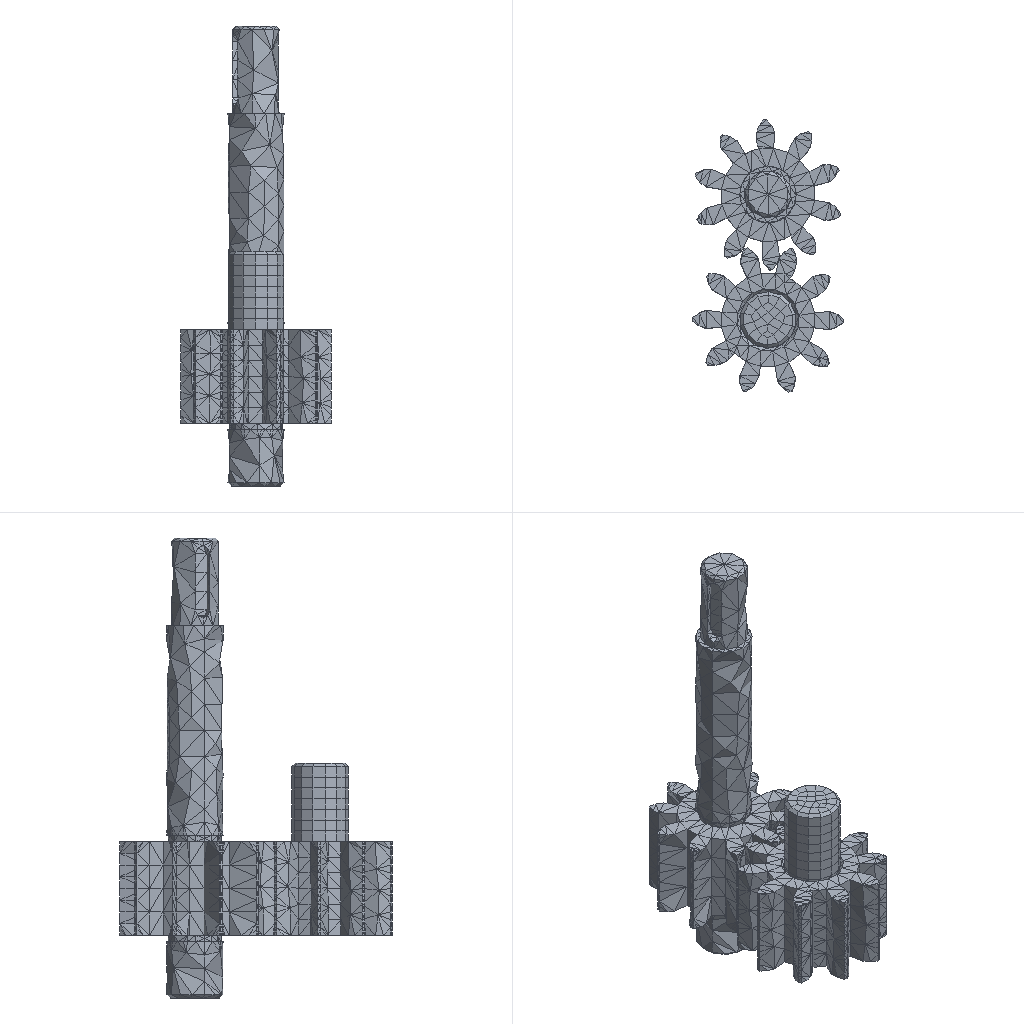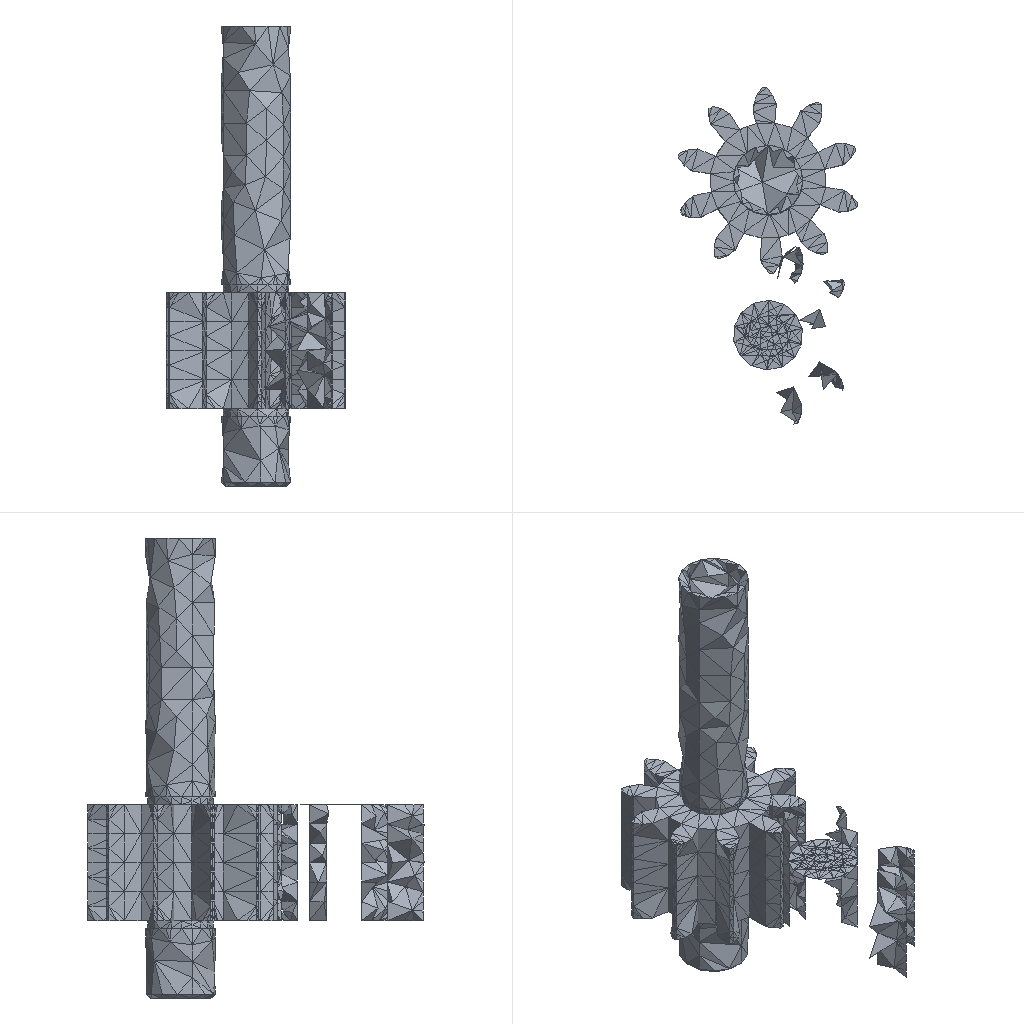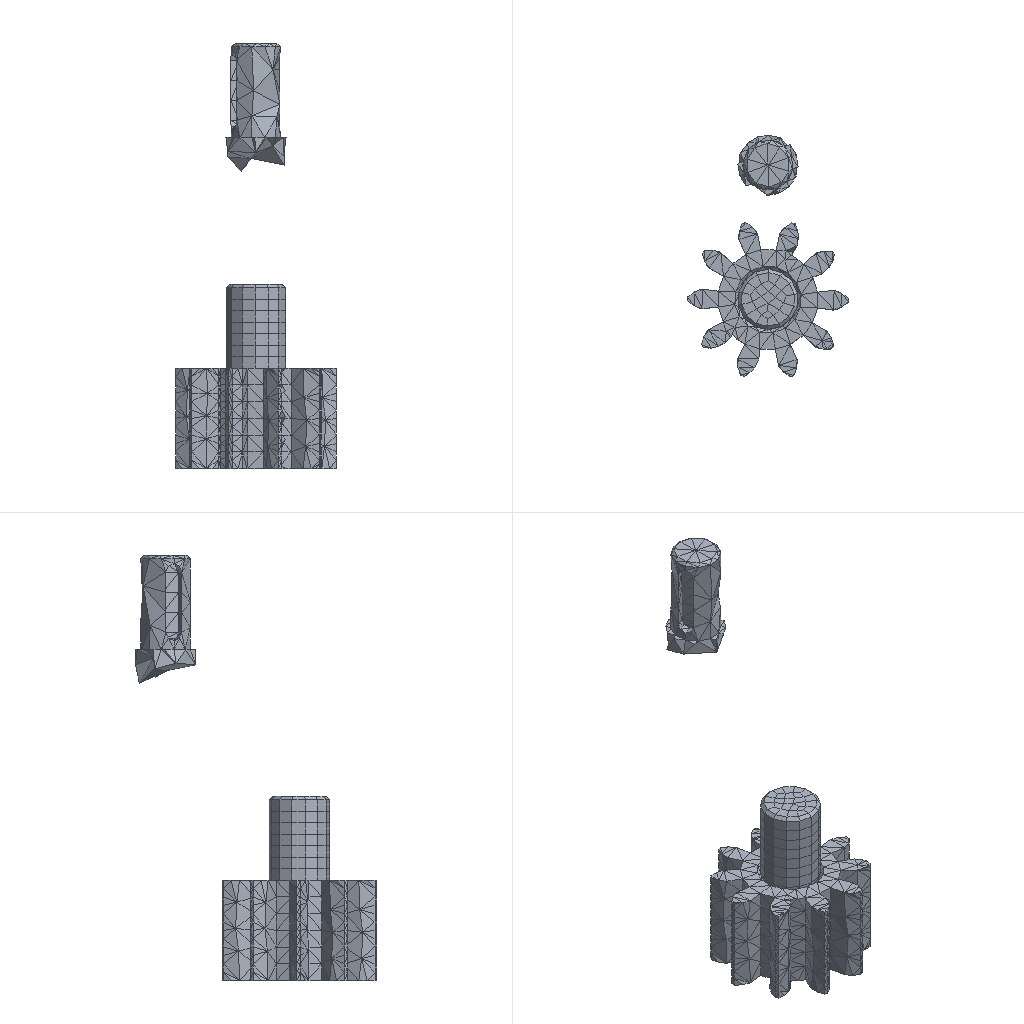Simulation study | ansys workbench
Set-up summary:
category,name,step,type,value,unit,region
solver,ansys_workbench
units,mm-N-s-tonne (MPa),,stated,"/units,MPA"
analysis,deck-1/LS1,,static
load_step,deck-1/LS1,deck-1/LS1,static,nsubst=1; time=1
analysis,deck-2/LS1,,modal,restart=True; perturbation=True; method=lanb; n_modes=6
load_step,deck-2/LS1,deck-2/LS1,modal
load_step,deck-2/LS1,deck-2/LS1,modal
mesh,deck-1.dat,,nodes,13194
mesh,deck-1.dat,,elements,7068
element_type,SOLID187,,,5473,,deck-1.dat
element_type,CONTA174,,,784,,deck-1.dat
element_type,SOLID186,,,443,,deck-1.dat
element_type,TARGE170,,,368,,deck-1.dat
mesh,deck-2.dat,,nodes,0
mesh,deck-2.dat,,elements,0
mesh,deck-2.dat,,note,"restart analysis: no node block, runs on the mesh of the upstream system's deck"
material,Structural Steel,,E,200000,tonne s^-2 mm^-1
material,Structural Steel,,nu,0.3
material,Structural Steel,,density,7.85e-09,tonne mm^-3
material,Structural Steel,,conductivity,60.5,tonne mm s^-3 C^-1
material,Structural Steel,,specific_heat,4.34e+08,mm^2 s^-2 C^-1
material,Structural Steel,,cte,1.2e-05,C^-1
material,Structural Steel,,permeability,10000
material,Structural Steel,,resistivity,0.00017,ohm mm
load,,deck-1/LS1,moment,"50000 [dir=(0, 0, 1) n=3]",,all
bc,Fixed Supports,deck-1/model,fixed,[dofs=ALL],,_FIXEDSU
contact,Contact Region,,bonded (always),element=CONTA174
contact,Contact Region 2,,bonded (always),element=CONTA174
contact,Contact Region 3,,bonded (always),element=CONTA174
contact,contact 4,,bonded (always),element=CONTA174
named_set,_CM49_FIXEDSU,,node,693
named_set,_FIXEDSU,,node,693
Results summary:
result,analyses[0].index,,,1
result,analyses[0].system,,,SYS
result,analyses[0].deck,,,deck-1.dat
result,analyses[0].solve_status,,,completed
result,analyses[0].analysis_type,,,static
result,analyses[0].physics,,,mechanical
result,analyses[0].unit_system,,,"NMM: mm, ton, N, s, mV, mA, degC"
result,analyses[0].n_sets,,,1
result,analyses[0].load_steps[0].set,set=1,,1
result,analyses[0].load_steps[0].time_or_freq,set=1,,1
result,analyses[0].load_steps[0].max_displacement_magnitude,set=1,,0.004698
result,analyses[0].load_steps[0].max_von_mises_nodal,set=1,,42.302
result,analyses[0].load_steps[0].reaction_force_sum_xyz[1],set=1,,-2.32875e-06
result,analyses[0].load_steps[0].reaction_force_sum_xyz[2],set=1,,7.38037e-06
result,analyses[0].load_steps[0].reaction_force_sum_xyz[3],set=1,,7.21953e-06
result,analyses[1].index,,,2
result,analyses[1].system,,,SYS-1
result,analyses[1].deck,,,deck-2.dat
result,analyses[1].solve_status,,,completed
result,analyses[1].analysis_type,,,modal
result,analyses[1].physics,,,mechanical
result,analyses[1].unit_system,,,"NMM: mm, ton, N, s, mV, mA, degC"
result,analyses[1].n_sets,,,6
result,analyses[1].modal_frequencies_hz[1],,,5626.54
result,analyses[1].modal_frequencies_hz[2],,,6709.81
result,analyses[1].modal_frequencies_hz[3],,,7467.24
result,analyses[1].modal_frequencies_hz[4],,,8337.49
result,analyses[1].modal_frequencies_hz[5],,,10993.6
result,analyses[1].modal_frequencies_hz[6],,,12668